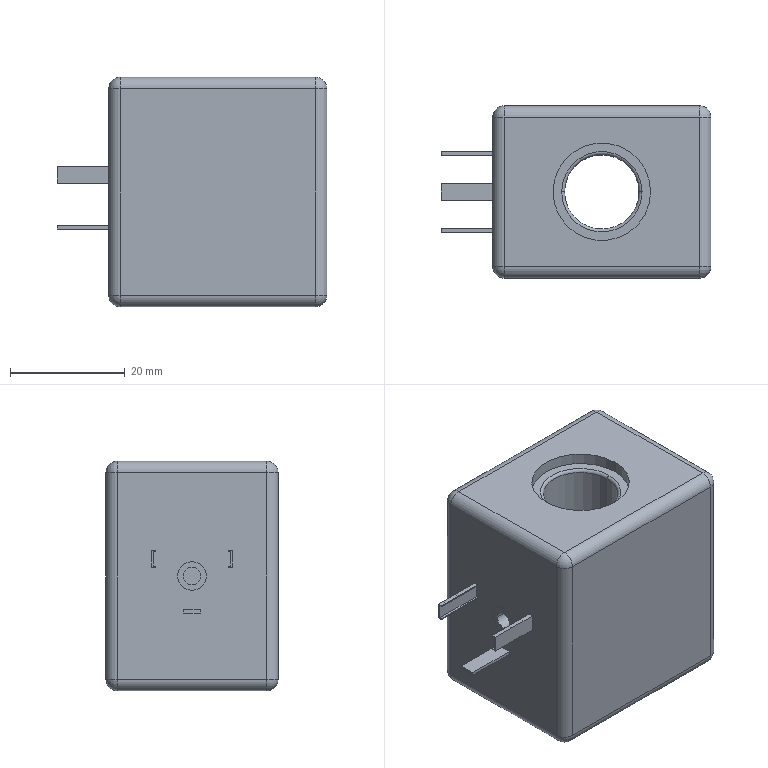Part | SolidWorks | features ICE 7, Fillet 2, Extrusion 1, MirrorPattern 1 | 1 solid | 70 faces | box 47 x 30 x 40 mm | volume 39521 mm3 | plane 34 | cylinder 24 | sphere 8 | torus 4 | commonest cylinder face diameters 4 x12 17 x4 3 x2 4.998 x2 5 x2 13 x2